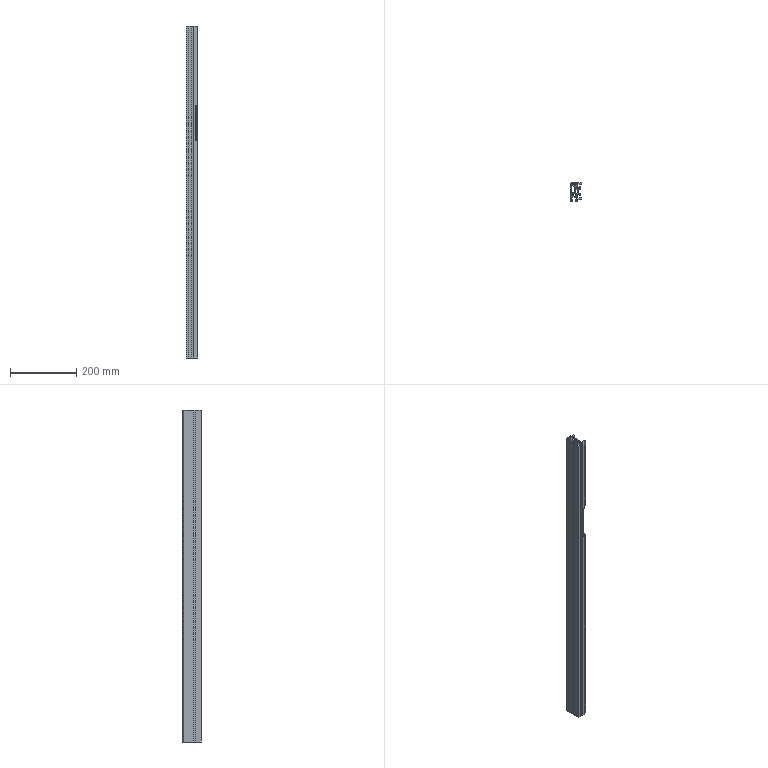Part | STEP file | PN_0001 Line Front Chain Guide Channel L1000 | 1 solid | 194 faces | box 35 x 55 x 1000 mm | volume 771293 mm3 | plane 148 | cylinder 37 | cone 9 | commonest cylinder face diameters 2.5 x9 2 x8 6.5 x6 2.3 x4 11 x4 24 x4